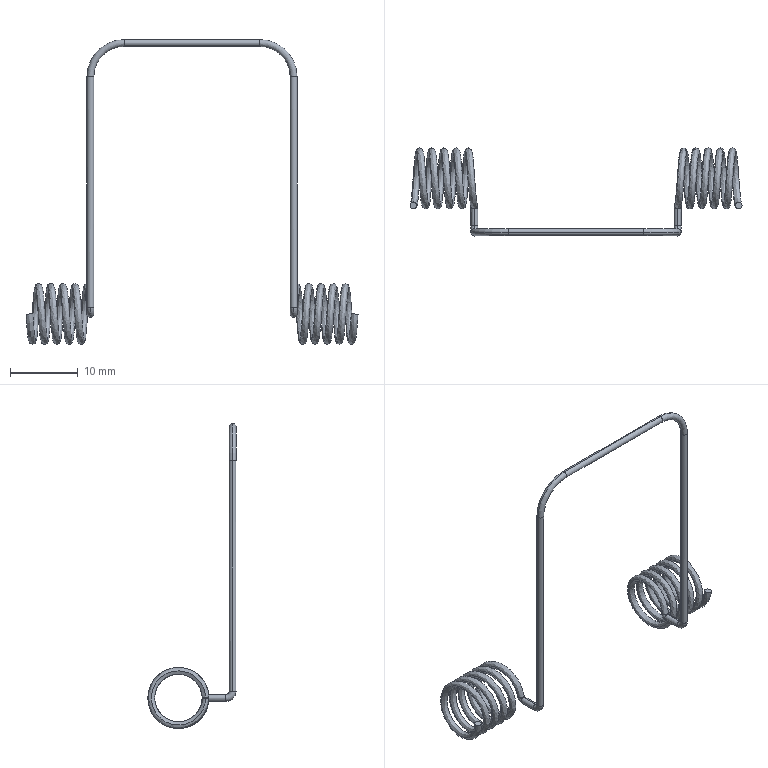Part | SolidWorks | features 3DProfileFeature 2, Helix 1, MirrorPattern 1, Sweep 1 | 1 solid | 30 faces | box 48.997 x 12.996 x 44.996 mm | volume 285.893 mm3 | cylinder 14 | torus 10 | spline 4 | plane 2 | commonest cylinder face diameters 1 x14